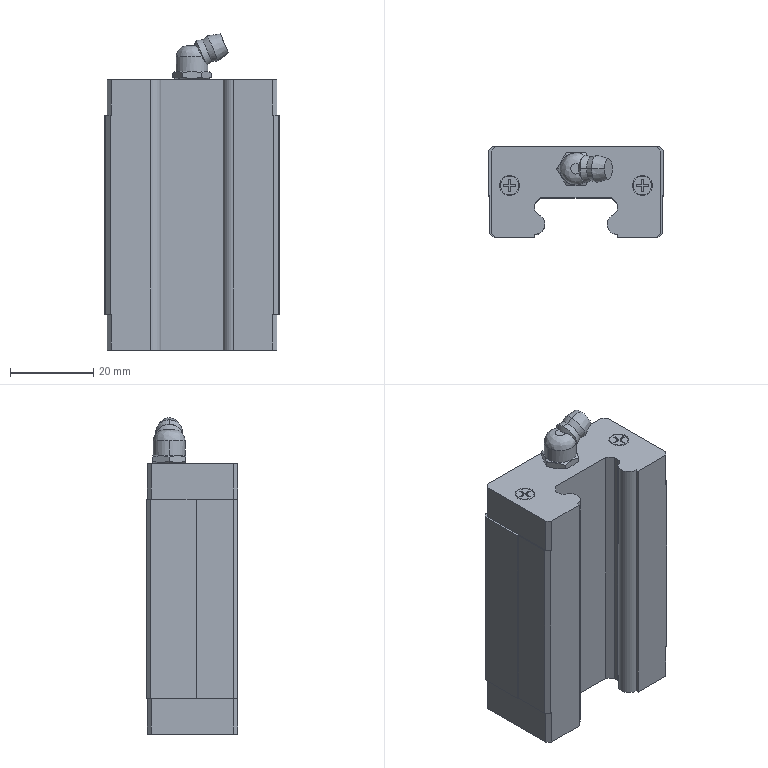Part | SolidWorks | features BaseBody 1 | 1 solid | 192 faces | box 42 x 22 x 76.2 mm | volume 48001 mm3 | plane 106 | cylinder 58 | cone 27 | spline 1 | commonest cylinder face diameters 3.08 x20 4.134 x8 4.4 x8 4.8 x8 9.2 x7 5 x3